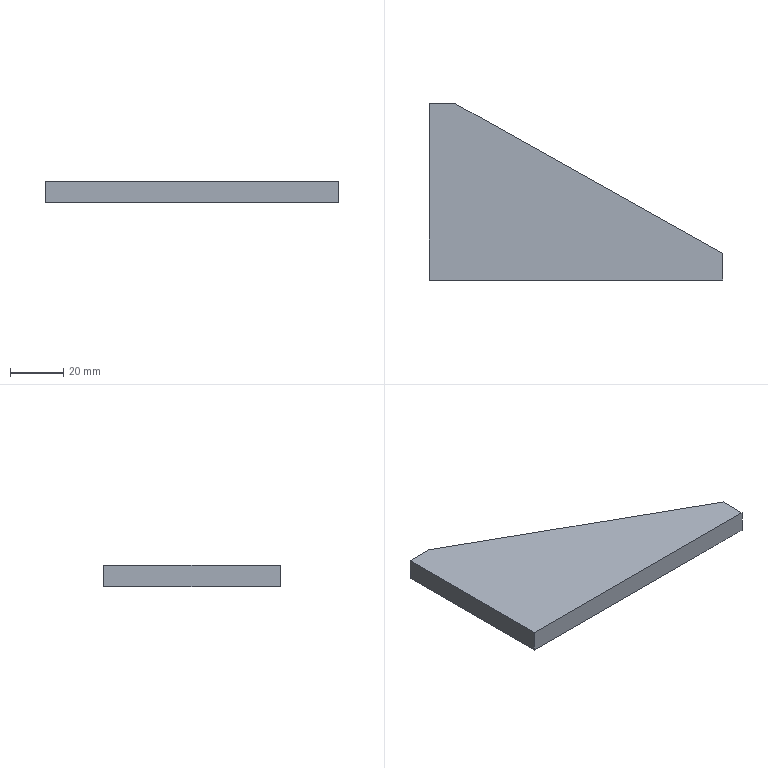Part | SolidWorks | features Extrusion 1 | 1 solid | 7 faces | box 110 x 66 x 8 mm | volume 35680 mm3 | plane 7
STEP:
#1=CARTESIAN_POINT('',(0.,66.,0.));
#2=VERTEX_POINT('',#1);
#3=CARTESIAN_POINT('',(0.,0.,0.));
#4=VERTEX_POINT('',#3);
#5=CARTESIAN_POINT('',(0.,0.,0.));
#6=DIRECTION('',(0.,-1.,0.));
#7=VECTOR('',#6,1000.);
#8=LINE('',#5,#7);
#9=EDGE_CURVE('',#2,#4,#8,.T.);
#10=ORIENTED_EDGE('',*,*,#9,.T.);
#11=CARTESIAN_POINT('',(0.,0.,8.));
#12=VERTEX_POINT('',#11);
#13=CARTESIAN_POINT('',(0.,0.,8.));
#14=DIRECTION('',(0.,0.,-1.));
#15=VECTOR('',#14,1000.);
#16=LINE('',#13,#15);
#17=EDGE_CURVE('',#12,#4,#16,.T.);
#18=ORIENTED_EDGE('',*,*,#17,.F.);
#19=CARTESIAN_POINT('',(0.,66.,8.));
#20=VERTEX_POINT('',#19);
#21=CARTESIAN_POINT('',(0.,0.,8.));
#22=DIRECTION('',(0.,-1.,0.));
#23=VECTOR('',#22,1000.);
#24=LINE('',#21,#23);
#25=EDGE_CURVE('',#20,#12,#24,.T.);
#26=ORIENTED_EDGE('',*,*,#25,.F.);
#27=CARTESIAN_POINT('',(0.,66.,8.));
#28=DIRECTION('',(0.,0.,-1.));
#29=VECTOR('',#28,1000.);
#30=LINE('',#27,#29);
#31=EDGE_CURVE('',#20,#2,#30,.T.);
#32=ORIENTED_EDGE('',*,*,#31,.T.);
#33=EDGE_LOOP('',(#10,#18,#26,#32));
#34=FACE_OUTER_BOUND('',#33,.T.);
#35=CARTESIAN_POINT('',(0.,0.,8.));
#36=DIRECTION('',(1.,0.,0.));
#37=DIRECTION('',(0.,0.,-1.));
#38=AXIS2_PLACEMENT_3D('',#35,#36,#37);
#39=PLANE('',#38);
#40=ADVANCED_FACE('',(#34),#39,.F.);
#41=CARTESIAN_POINT('',(110.,0.,0.));
#42=VERTEX_POINT('',#41);
#43=CARTESIAN_POINT('',(0.,0.,0.));
#44=DIRECTION('',(1.,0.,0.));
#45=VECTOR('',#44,1000.);
#46=LINE('',#43,#45);
#47=EDGE_CURVE('',#4,#42,#46,.T.);
#48=ORIENTED_EDGE('',*,*,#47,.T.);
#49=CARTESIAN_POINT('',(110.,0.,8.));
#50=VERTEX_POINT('',#49);
#51=CARTESIAN_POINT('',(110.,0.,8.));
#52=DIRECTION('',(0.,0.,-1.));
#53=VECTOR('',#52,1000.);
#54=LINE('',#51,#53);
#55=EDGE_CURVE('',#50,#42,#54,.T.);
#56=ORIENTED_EDGE('',*,*,#55,.F.);
#57=CARTESIAN_POINT('',(0.,0.,8.));
#58=DIRECTION('',(1.,0.,0.));
#59=VECTOR('',#58,1000.);
#60=LINE('',#57,#59);
#61=EDGE_CURVE('',#12,#50,#60,.T.);
#62=ORIENTED_EDGE('',*,*,#61,.F.);
#63=ORIENTED_EDGE('',*,*,#17,.T.);
#64=EDGE_LOOP('',(#48,#56,#62,#63));
#65=FACE_OUTER_BOUND('',#64,.T.);
#66=CARTESIAN_POINT('',(0.,0.,8.));
#67=DIRECTION('',(0.,1.,0.));
#68=DIRECTION('',(0.,0.,1.));
#69=AXIS2_PLACEMENT_3D('',#66,#67,#68);
#70=PLANE('',#69);
#71=ADVANCED_FACE('',(#65),#70,.F.);
#72=CARTESIAN_POINT('',(110.,10.,0.));
#73=VERTEX_POINT('',#72);
#74=CARTESIAN_POINT('',(110.,0.,0.));
#75=DIRECTION('',(0.,1.,0.));
#76=VECTOR('',#75,1000.);
#77=LINE('',#74,#76);
#78=EDGE_CURVE('',#42,#73,#77,.T.);
#79=ORIENTED_EDGE('',*,*,#78,.T.);
#80=CARTESIAN_POINT('',(110.,10.,8.));
#81=VERTEX_POINT('',#80);
#82=CARTESIAN_POINT('',(110.,10.,8.));
#83=DIRECTION('',(0.,0.,-1.));
#84=VECTOR('',#83,1000.);
#85=LINE('',#82,#84);
#86=EDGE_CURVE('',#81,#73,#85,.T.);
#87=ORIENTED_EDGE('',*,*,#86,.F.);
#88=CARTESIAN_POINT('',(110.,0.,8.));
#89=DIRECTION('',(0.,1.,0.));
#90=VECTOR('',#89,1000.);
#91=LINE('',#88,#90);
#92=EDGE_CURVE('',#50,#81,#91,.T.);
#93=ORIENTED_EDGE('',*,*,#92,.F.);
#94=ORIENTED_EDGE('',*,*,#55,.T.);
#95=EDGE_LOOP('',(#79,#87,#93,#94));
#96=FACE_OUTER_BOUND('',#95,.T.);
#97=CARTESIAN_POINT('',(110.,0.,8.));
#98=DIRECTION('',(-1.,0.,0.));
#99=DIRECTION('',(0.,0.,1.));
#100=AXIS2_PLACEMENT_3D('',#97,#98,#99);
#101=PLANE('',#100);
#102=ADVANCED_FACE('',(#96),#101,.F.);
#103=CARTESIAN_POINT('',(10.,66.,0.));
#104=VERTEX_POINT('',#103);
#105=CARTESIAN_POINT('',(10.,66.,0.));
#106=DIRECTION('',(-0.8725,0.4886,0.));
#107=VECTOR('',#106,1000.);
#108=LINE('',#105,#107);
#109=EDGE_CURVE('',#73,#104,#108,.T.);
#110=ORIENTED_EDGE('',*,*,#109,.T.);
#111=CARTESIAN_POINT('',(10.,66.,8.));
#112=VERTEX_POINT('',#111);
#113=CARTESIAN_POINT('',(10.,66.,8.));
#114=DIRECTION('',(0.,0.,-1.));
#115=VECTOR('',#114,1000.);
#116=LINE('',#113,#115);
#117=EDGE_CURVE('',#112,#104,#116,.T.);
#118=ORIENTED_EDGE('',*,*,#117,.F.);
#119=CARTESIAN_POINT('',(10.,66.,8.));
#120=DIRECTION('',(-0.8725,0.4886,0.));
#121=VECTOR('',#120,1000.);
#122=LINE('',#119,#121);
#123=EDGE_CURVE('',#81,#112,#122,.T.);
#124=ORIENTED_EDGE('',*,*,#123,.F.);
#125=ORIENTED_EDGE('',*,*,#86,.T.);
#126=EDGE_LOOP('',(#110,#118,#124,#125));
#127=FACE_OUTER_BOUND('',#126,.T.);
#128=CARTESIAN_POINT('',(10.,66.,8.));
#129=DIRECTION('',(-0.4886,-0.8725,0.));
#130=DIRECTION('',(0.8725,-0.4886,0.));
#131=AXIS2_PLACEMENT_3D('',#128,#129,#130);
#132=PLANE('',#131);
#133=ADVANCED_FACE('',(#127),#132,.F.);
#134=CARTESIAN_POINT('',(0.,66.,0.));
#135=DIRECTION('',(-1.,0.,0.));
#136=VECTOR('',#135,1000.);
#137=LINE('',#134,#136);
#138=EDGE_CURVE('',#104,#2,#137,.T.);
#139=ORIENTED_EDGE('',*,*,#138,.T.);
#140=ORIENTED_EDGE('',*,*,#31,.F.);
#141=CARTESIAN_POINT('',(0.,66.,8.));
#142=DIRECTION('',(-1.,0.,0.));
#143=VECTOR('',#142,1000.);
#144=LINE('',#141,#143);
#145=EDGE_CURVE('',#112,#20,#144,.T.);
#146=ORIENTED_EDGE('',*,*,#145,.F.);
#147=ORIENTED_EDGE('',*,*,#117,.T.);
#148=EDGE_LOOP('',(#139,#140,#146,#147));
#149=FACE_OUTER_BOUND('',#148,.T.);
#150=CARTESIAN_POINT('',(0.,66.,8.));
#151=DIRECTION('',(0.,-1.,0.));
#152=DIRECTION('',(0.,0.,-1.));
#153=AXIS2_PLACEMENT_3D('',#150,#151,#152);
#154=PLANE('',#153);
#155=ADVANCED_FACE('',(#149),#154,.F.);
#156=ORIENTED_EDGE('',*,*,#25,.T.);
#157=ORIENTED_EDGE('',*,*,#61,.T.);
#158=ORIENTED_EDGE('',*,*,#92,.T.);
#159=ORIENTED_EDGE('',*,*,#123,.T.);
#160=ORIENTED_EDGE('',*,*,#145,.T.);
#161=EDGE_LOOP('',(#156,#157,#158,#159,#160));
#162=FACE_OUTER_BOUND('',#161,.T.);
#163=CARTESIAN_POINT('',(0.,0.,8.));
#164=DIRECTION('',(0.,0.,-1.));
#165=DIRECTION('',(-1.,0.,0.));
#166=AXIS2_PLACEMENT_3D('',#163,#164,#165);
#167=PLANE('',#166);
#168=ADVANCED_FACE('',(#162),#167,.F.);
#169=ORIENTED_EDGE('',*,*,#9,.F.);
#170=ORIENTED_EDGE('',*,*,#138,.F.);
#171=ORIENTED_EDGE('',*,*,#109,.F.);
#172=ORIENTED_EDGE('',*,*,#78,.F.);
#173=ORIENTED_EDGE('',*,*,#47,.F.);
#174=EDGE_LOOP('',(#169,#170,#171,#172,#173));
#175=FACE_OUTER_BOUND('',#174,.T.);
#176=CARTESIAN_POINT('',(0.,0.,0.));
#177=DIRECTION('',(0.,0.,-1.));
#178=DIRECTION('',(-1.,0.,0.));
#179=AXIS2_PLACEMENT_3D('',#176,#177,#178);
#180=PLANE('',#179);
#181=ADVANCED_FACE('',(#175),#180,.T.);
#182=CLOSED_SHELL('',(#40,#71,#102,#133,#155,#168,#181));
#183=MANIFOLD_SOLID_BREP('',#182);
#184=CARTESIAN_POINT('',(0.,0.,0.));
#185=DIRECTION('',(0.,0.,1.));
#186=DIRECTION('',(1.,0.,0.));
#187=AXIS2_PLACEMENT_3D('',#184,#185,#186);
#188=(LENGTH_UNIT()NAMED_UNIT(*)SI_UNIT(.MILLI.,.METRE.));
#189=UNCERTAINTY_MEASURE_WITH_UNIT(LENGTH_MEASURE(0.00001),#188,'','');
#190=(NAMED_UNIT(*)PLANE_ANGLE_UNIT()SI_UNIT($,.RADIAN.));
#191=(NAMED_UNIT(*)SI_UNIT($,.STERADIAN.)SOLID_ANGLE_UNIT());
#192=(GEOMETRIC_REPRESENTATION_CONTEXT(3)GLOBAL_UNCERTAINTY_ASSIGNED_CONTEXT((#189))GLOBAL_UNIT_ASSIGNED_CONTEXT((#188,#190,#191))REPRESENTATION_CONTEXT('',''));
#193=ADVANCED_BREP_SHAPE_REPRESENTATION('',(#183,#187),#192);